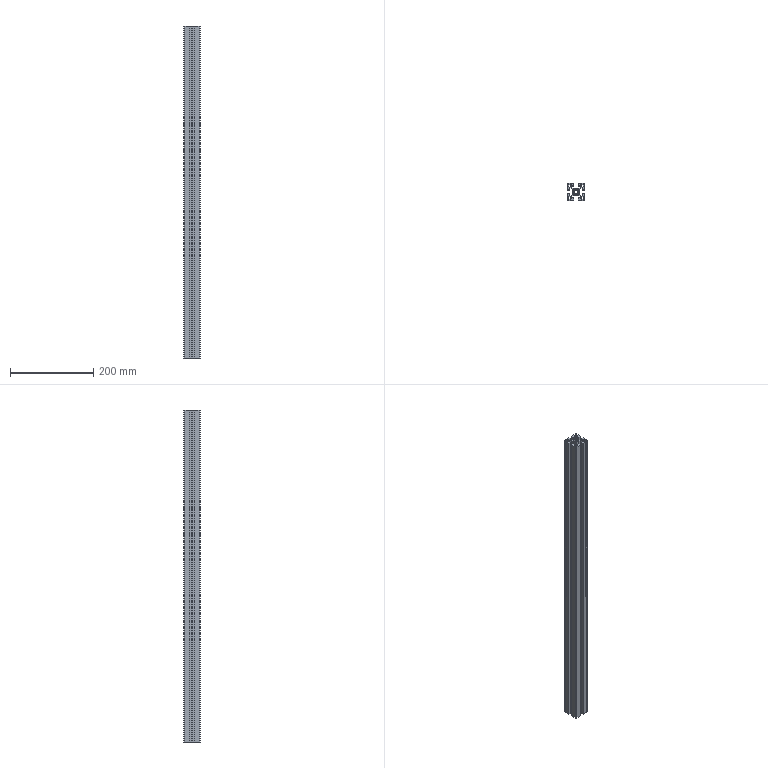Part | STEP file | 1.6米HFS8-4040-110 | 1 solid | 111 faces | box 40 x 40 x 800 mm | volume 497640 mm3 | plane 74 | cylinder 37 | commonest cylinder face diameters 2 x28 10.5 x5 6 x4